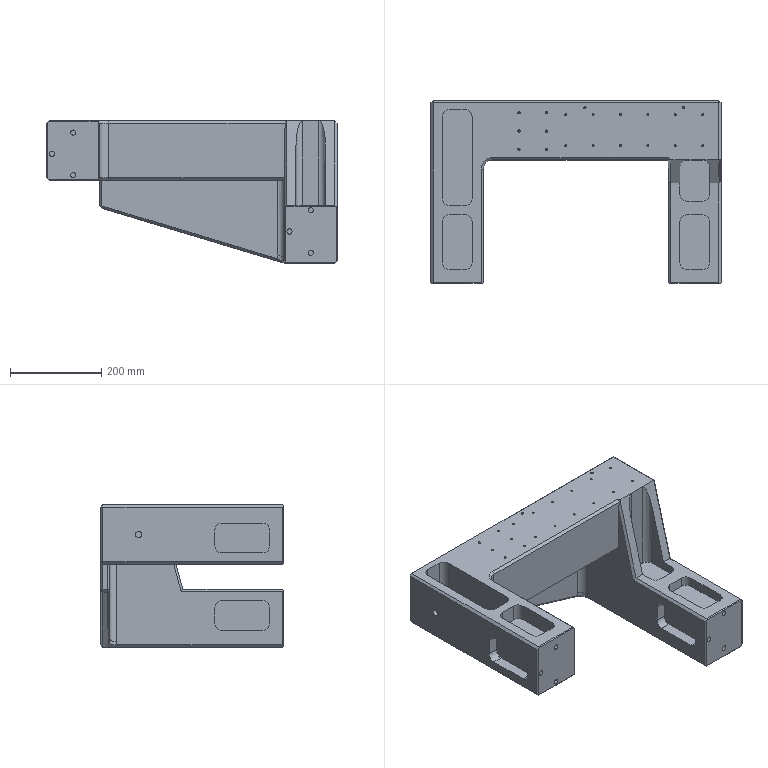Part | STEP file | SOLID | 1 solid | 344 faces | box 635 x 400 x 312 mm | volume 15425228 mm3 | cylinder 149 | plane 117 | cone 77 | spline 1 | commonest cylinder face diameters 30 x56 4.2 x28 5 x20 2.5 x16 3.3 x12 11.5 x12